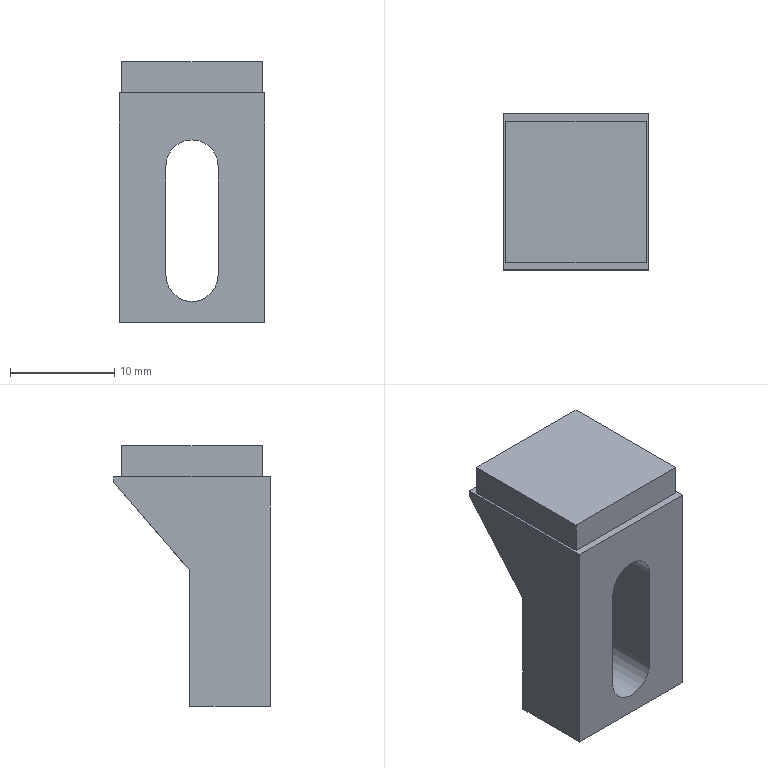Part | SolidWorks | features ICE 4, Extrusion 1 | 1 solid | 24 faces | box 14 x 15 x 25 mm | volume 2645 mm3 | plane 18 | cylinder 6 | commonest cylinder face diameters 5 x3 8.5 x3
STEP:
#1=CARTESIAN_POINT('',(0.,-7.5,-6.));
#2=VERTEX_POINT('',#1);
#3=CARTESIAN_POINT('',(2.5,-7.5,-8.5));
#4=VERTEX_POINT('',#3);
#5=CARTESIAN_POINT('',(0.,-7.5,-8.5));
#6=DIRECTION('',(0.,1.,0.));
#7=DIRECTION('',(0.,0.,1.));
#8=AXIS2_PLACEMENT_3D('',#5,#6,#7);
#9=CIRCLE('',#8,2.5);
#10=EDGE_CURVE('',#2,#4,#9,.T.);
#11=ORIENTED_EDGE('',*,*,#10,.F.);
#12=CARTESIAN_POINT('',(0.,-1.1,-6.));
#13=VERTEX_POINT('',#12);
#14=CARTESIAN_POINT('',(0.,-11.1,-6.));
#15=DIRECTION('',(0.,1.,0.));
#16=VECTOR('',#15,1000.);
#17=LINE('',#14,#16);
#18=EDGE_CURVE('',#2,#13,#17,.T.);
#19=ORIENTED_EDGE('',*,*,#18,.T.);
#20=CARTESIAN_POINT('',(2.5,-1.1,-8.5));
#21=VERTEX_POINT('',#20);
#22=CARTESIAN_POINT('',(0.,-1.1,-8.5));
#23=DIRECTION('',(0.,-1.,0.));
#24=DIRECTION('',(0.,0.,-1.));
#25=AXIS2_PLACEMENT_3D('',#22,#23,#24);
#26=CIRCLE('',#25,2.5);
#27=EDGE_CURVE('',#21,#13,#26,.T.);
#28=ORIENTED_EDGE('',*,*,#27,.F.);
#29=CARTESIAN_POINT('',(2.5,-11.1,-8.5));
#30=DIRECTION('',(0.,1.,0.));
#31=VECTOR('',#30,1000.);
#32=LINE('',#29,#31);
#33=EDGE_CURVE('',#4,#21,#32,.T.);
#34=ORIENTED_EDGE('',*,*,#33,.F.);
#35=EDGE_LOOP('',(#11,#19,#28,#34));
#36=FACE_OUTER_BOUND('',#35,.T.);
#37=CARTESIAN_POINT('',(0.,-11.1,-8.5));
#38=DIRECTION('',(0.,1.,0.));
#39=DIRECTION('',(0.,0.,1.));
#40=AXIS2_PLACEMENT_3D('',#37,#38,#39);
#41=CYLINDRICAL_SURFACE('',#40,2.5);
#42=ADVANCED_FACE('',(#36),#41,.F.);
#43=CARTESIAN_POINT('',(0.,-1.1,-4.25));
#44=VERTEX_POINT('',#43);
#45=CARTESIAN_POINT('',(4.25,-1.1,-8.5));
#46=VERTEX_POINT('',#45);
#47=CARTESIAN_POINT('',(0.,-1.1,-8.5));
#48=DIRECTION('',(0.,1.,0.));
#49=DIRECTION('',(0.,0.,-1.));
#50=AXIS2_PLACEMENT_3D('',#47,#48,#49);
#51=CIRCLE('',#50,4.25);
#52=EDGE_CURVE('',#44,#46,#51,.T.);
#53=ORIENTED_EDGE('',*,*,#52,.F.);
#54=CARTESIAN_POINT('',(0.,5.568,-4.25));
#55=VERTEX_POINT('',#54);
#56=CARTESIAN_POINT('',(0.,-23.215,-4.25));
#57=DIRECTION('',(0.,1.,0.));
#58=VECTOR('',#57,1000.);
#59=LINE('',#56,#58);
#60=EDGE_CURVE('',#44,#55,#59,.T.);
#61=ORIENTED_EDGE('',*,*,#60,.T.);
#62=CARTESIAN_POINT('',(4.25,1.918,-8.5));
#63=VERTEX_POINT('',#62);
#64=CARTESIAN_POINT('',(4.25,1.918,-8.5));
#65=CARTESIAN_POINT('',(4.25,4.056,-6.01));
#66=CARTESIAN_POINT('',(2.49,5.568,-4.25));
#67=CARTESIAN_POINT('',(0.,5.568,-4.25));
#68=(BOUNDED_CURVE()B_SPLINE_CURVE(3,(#64,#65,#66,#67),.UNSPECIFIED.,.F.,.F.)B_SPLINE_CURVE_WITH_KNOTS((4,4),(4.712,6.283),.UNSPECIFIED.)CURVE()GEOMETRIC_REPRESENTATION_ITEM()RATIONAL_B_SPLINE_CURVE((1.,0.8047,0.8047,1.))REPRESENTATION_ITEM(''));
#69=EDGE_CURVE('',#63,#55,#68,.T.);
#70=ORIENTED_EDGE('',*,*,#69,.F.);
#71=CARTESIAN_POINT('',(4.25,-23.215,-8.5));
#72=DIRECTION('',(0.,1.,0.));
#73=VECTOR('',#72,1000.);
#74=LINE('',#71,#73);
#75=EDGE_CURVE('',#46,#63,#74,.T.);
#76=ORIENTED_EDGE('',*,*,#75,.F.);
#77=EDGE_LOOP('',(#53,#61,#70,#76));
#78=FACE_OUTER_BOUND('',#77,.T.);
#79=CARTESIAN_POINT('',(0.,-23.215,-8.5));
#80=DIRECTION('',(0.,1.,0.));
#81=DIRECTION('',(0.,0.,1.));
#82=AXIS2_PLACEMENT_3D('',#79,#80,#81);
#83=CYLINDRICAL_SURFACE('',#82,4.25);
#84=ADVANCED_FACE('',(#78),#83,.F.);
#85=CARTESIAN_POINT('',(6.75,-6.75,-1.5));
#86=VERTEX_POINT('',#85);
#87=CARTESIAN_POINT('',(6.75,6.75,-1.5));
#88=VERTEX_POINT('',#87);
#89=CARTESIAN_POINT('',(6.75,6.75,-1.5));
#90=DIRECTION('',(0.,1.,0.));
#91=VECTOR('',#90,1000.);
#92=LINE('',#89,#91);
#93=EDGE_CURVE('',#86,#88,#92,.T.);
#94=ORIENTED_EDGE('',*,*,#93,.T.);
#95=CARTESIAN_POINT('',(6.75,6.75,1.5));
#96=VERTEX_POINT('',#95);
#97=CARTESIAN_POINT('',(6.75,6.75,1.5));
#98=DIRECTION('',(0.,0.,-1.));
#99=VECTOR('',#98,1000.);
#100=LINE('',#97,#99);
#101=EDGE_CURVE('',#96,#88,#100,.T.);
#102=ORIENTED_EDGE('',*,*,#101,.F.);
#103=CARTESIAN_POINT('',(6.75,-6.75,1.5));
#104=VERTEX_POINT('',#103);
#105=CARTESIAN_POINT('',(6.75,6.75,1.5));
#106=DIRECTION('',(0.,1.,0.));
#107=VECTOR('',#106,1000.);
#108=LINE('',#105,#107);
#109=EDGE_CURVE('',#104,#96,#108,.T.);
#110=ORIENTED_EDGE('',*,*,#109,.F.);
#111=CARTESIAN_POINT('',(6.75,-6.75,1.5));
#112=DIRECTION('',(0.,0.,-1.));
#113=VECTOR('',#112,1000.);
#114=LINE('',#111,#113);
#115=EDGE_CURVE('',#104,#86,#114,.T.);
#116=ORIENTED_EDGE('',*,*,#115,.T.);
#117=EDGE_LOOP('',(#94,#102,#110,#116));
#118=FACE_OUTER_BOUND('',#117,.T.);
#119=CARTESIAN_POINT('',(6.75,6.75,1.5));
#120=DIRECTION('',(-1.,0.,0.));
#121=DIRECTION('',(0.,0.,1.));
#122=AXIS2_PLACEMENT_3D('',#119,#120,#121);
#123=PLANE('',#122);
#124=ADVANCED_FACE('',(#118),#123,.F.);
#125=CARTESIAN_POINT('',(-6.75,6.75,-1.5));
#126=VERTEX_POINT('',#125);
#127=CARTESIAN_POINT('',(-6.75,6.75,-1.5));
#128=DIRECTION('',(-1.,0.,0.));
#129=VECTOR('',#128,1000.);
#130=LINE('',#127,#129);
#131=EDGE_CURVE('',#88,#126,#130,.T.);
#132=ORIENTED_EDGE('',*,*,#131,.T.);
#133=CARTESIAN_POINT('',(-6.75,6.75,1.5));
#134=VERTEX_POINT('',#133);
#135=CARTESIAN_POINT('',(-6.75,6.75,1.5));
#136=DIRECTION('',(0.,0.,-1.));
#137=VECTOR('',#136,1000.);
#138=LINE('',#135,#137);
#139=EDGE_CURVE('',#134,#126,#138,.T.);
#140=ORIENTED_EDGE('',*,*,#139,.F.);
#141=CARTESIAN_POINT('',(-6.75,6.75,1.5));
#142=DIRECTION('',(-1.,0.,0.));
#143=VECTOR('',#142,1000.);
#144=LINE('',#141,#143);
#145=EDGE_CURVE('',#96,#134,#144,.T.);
#146=ORIENTED_EDGE('',*,*,#145,.F.);
#147=ORIENTED_EDGE('',*,*,#101,.T.);
#148=EDGE_LOOP('',(#132,#140,#146,#147));
#149=FACE_OUTER_BOUND('',#148,.T.);
#150=CARTESIAN_POINT('',(-6.75,6.75,1.5));
#151=DIRECTION('',(0.,-1.,0.));
#152=DIRECTION('',(0.,0.,-1.));
#153=AXIS2_PLACEMENT_3D('',#150,#151,#152);
#154=PLANE('',#153);
#155=ADVANCED_FACE('',(#149),#154,.F.);
#156=CARTESIAN_POINT('',(-6.75,-6.75,-1.5));
#157=VERTEX_POINT('',#156);
#158=CARTESIAN_POINT('',(-6.75,6.75,-1.5));
#159=DIRECTION('',(0.,-1.,0.));
#160=VECTOR('',#159,1000.);
#161=LINE('',#158,#160);
#162=EDGE_CURVE('',#126,#157,#161,.T.);
#163=ORIENTED_EDGE('',*,*,#162,.T.);
#164=CARTESIAN_POINT('',(-6.75,-6.75,1.5));
#165=VERTEX_POINT('',#164);
#166=CARTESIAN_POINT('',(-6.75,-6.75,1.5));
#167=DIRECTION('',(0.,0.,-1.));
#168=VECTOR('',#167,1000.);
#169=LINE('',#166,#168);
#170=EDGE_CURVE('',#165,#157,#169,.T.);
#171=ORIENTED_EDGE('',*,*,#170,.F.);
#172=CARTESIAN_POINT('',(-6.75,6.75,1.5));
#173=DIRECTION('',(0.,-1.,0.));
#174=VECTOR('',#173,1000.);
#175=LINE('',#172,#174);
#176=EDGE_CURVE('',#134,#165,#175,.T.);
#177=ORIENTED_EDGE('',*,*,#176,.F.);
#178=ORIENTED_EDGE('',*,*,#139,.T.);
#179=EDGE_LOOP('',(#163,#171,#177,#178));
#180=FACE_OUTER_BOUND('',#179,.T.);
#181=CARTESIAN_POINT('',(-6.75,6.75,1.5));
#182=DIRECTION('',(1.,0.,0.));
#183=DIRECTION('',(0.,0.,-1.));
#184=AXIS2_PLACEMENT_3D('',#181,#182,#183);
#185=PLANE('',#184);
#186=ADVANCED_FACE('',(#180),#185,.F.);
#187=CARTESIAN_POINT('',(-6.75,-6.75,-1.5));
#188=DIRECTION('',(1.,0.,0.));
#189=VECTOR('',#188,1000.);
#190=LINE('',#187,#189);
#191=EDGE_CURVE('',#157,#86,#190,.T.);
#192=ORIENTED_EDGE('',*,*,#191,.T.);
#193=ORIENTED_EDGE('',*,*,#115,.F.);
#194=CARTESIAN_POINT('',(-6.75,-6.75,1.5));
#195=DIRECTION('',(1.,0.,0.));
#196=VECTOR('',#195,1000.);
#197=LINE('',#194,#196);
#198=EDGE_CURVE('',#165,#104,#197,.T.);
#199=ORIENTED_EDGE('',*,*,#198,.F.);
#200=ORIENTED_EDGE('',*,*,#170,.T.);
#201=EDGE_LOOP('',(#192,#193,#199,#200));
#202=FACE_OUTER_BOUND('',#201,.T.);
#203=CARTESIAN_POINT('',(-6.75,-6.75,1.5));
#204=DIRECTION('',(0.,1.,0.));
#205=DIRECTION('',(0.,0.,1.));
#206=AXIS2_PLACEMENT_3D('',#203,#204,#205);
#207=PLANE('',#206);
#208=ADVANCED_FACE('',(#202),#207,.F.);
#209=ORIENTED_EDGE('',*,*,#109,.T.);
#210=ORIENTED_EDGE('',*,*,#145,.T.);
#211=ORIENTED_EDGE('',*,*,#176,.T.);
#212=ORIENTED_EDGE('',*,*,#198,.T.);
#213=EDGE_LOOP('',(#209,#210,#211,#212));
#214=FACE_OUTER_BOUND('',#213,.T.);
#215=CARTESIAN_POINT('',(0.,0.,1.5));
#216=DIRECTION('',(0.,0.,1.));
#217=DIRECTION('',(1.,0.,0.));
#218=AXIS2_PLACEMENT_3D('',#215,#216,#217);
#219=PLANE('',#218);
#220=ADVANCED_FACE('',(#214),#219,.T.);
#221=CARTESIAN_POINT('',(-7.,-7.5,-1.5));
#222=VERTEX_POINT('',#221);
#223=CARTESIAN_POINT('',(-7.,7.5,-1.5));
#224=VERTEX_POINT('',#223);
#225=CARTESIAN_POINT('',(-7.,7.5,-1.5));
#226=DIRECTION('',(0.,1.,0.));
#227=VECTOR('',#226,1000.);
#228=LINE('',#225,#227);
#229=EDGE_CURVE('',#222,#224,#228,.T.);
#230=ORIENTED_EDGE('',*,*,#229,.F.);
#231=CARTESIAN_POINT('',(7.,-7.5,-1.5));
#232=VERTEX_POINT('',#231);
#233=CARTESIAN_POINT('',(7.,-7.5,-1.5));
#234=DIRECTION('',(-1.,0.,0.));
#235=VECTOR('',#234,1000.);
#236=LINE('',#233,#235);
#237=EDGE_CURVE('',#232,#222,#236,.T.);
#238=ORIENTED_EDGE('',*,*,#237,.F.);
#239=CARTESIAN_POINT('',(7.,7.5,-1.5));
#240=VERTEX_POINT('',#239);
#241=CARTESIAN_POINT('',(7.,7.5,-1.5));
#242=DIRECTION('',(0.,-1.,0.));
#243=VECTOR('',#242,1000.);
#244=LINE('',#241,#243);
#245=EDGE_CURVE('',#240,#232,#244,.T.);
#246=ORIENTED_EDGE('',*,*,#245,.F.);
#247=CARTESIAN_POINT('',(7.,7.5,-1.5));
#248=DIRECTION('',(1.,0.,0.));
#249=VECTOR('',#248,1000.);
#250=LINE('',#247,#249);
#251=EDGE_CURVE('',#224,#240,#250,.T.);
#252=ORIENTED_EDGE('',*,*,#251,.F.);
#253=EDGE_LOOP('',(#230,#238,#246,#252));
#254=FACE_OUTER_BOUND('',#253,.T.);
#255=ORIENTED_EDGE('',*,*,#131,.F.);
#256=ORIENTED_EDGE('',*,*,#93,.F.);
#257=ORIENTED_EDGE('',*,*,#191,.F.);
#258=ORIENTED_EDGE('',*,*,#162,.F.);
#259=EDGE_LOOP('',(#255,#256,#257,#258));
#260=FACE_BOUND('',#259,.T.);
#261=CARTESIAN_POINT('',(0.,0.,-1.5));
#262=DIRECTION('',(0.,0.,-1.));
#263=DIRECTION('',(-1.,0.,0.));
#264=AXIS2_PLACEMENT_3D('',#261,#262,#263);
#265=PLANE('',#264);
#266=ADVANCED_FACE('',(#254,#260),#265,.F.);
#267=CARTESIAN_POINT('',(-7.,7.5,-2.));
#268=VERTEX_POINT('',#267);
#269=CARTESIAN_POINT('',(-7.,0.2,-10.5));
#270=VERTEX_POINT('',#269);
#271=CARTESIAN_POINT('',(-7.,-3.127,-14.374));
#272=DIRECTION('',(0.,-0.6515,-0.7586));
#273=VECTOR('',#272,1000.);
#274=LINE('',#271,#273);
#275=EDGE_CURVE('',#268,#270,#274,.T.);
#276=ORIENTED_EDGE('',*,*,#275,.T.);
#277=CARTESIAN_POINT('',(-7.,0.2,-23.5));
#278=VERTEX_POINT('',#277);
#279=CARTESIAN_POINT('',(-7.,0.2,-23.5));
#280=DIRECTION('',(0.,0.,-1.));
#281=VECTOR('',#280,1000.);
#282=LINE('',#279,#281);
#283=EDGE_CURVE('',#270,#278,#282,.T.);
#284=ORIENTED_EDGE('',*,*,#283,.T.);
#285=CARTESIAN_POINT('',(-7.,-7.5,-23.5));
#286=VERTEX_POINT('',#285);
#287=CARTESIAN_POINT('',(-7.,7.5,-23.5));
#288=DIRECTION('',(0.,1.,0.));
#289=VECTOR('',#288,1000.);
#290=LINE('',#287,#289);
#291=EDGE_CURVE('',#286,#278,#290,.T.);
#292=ORIENTED_EDGE('',*,*,#291,.F.);
#293=CARTESIAN_POINT('',(-7.,-7.5,-23.5));
#294=DIRECTION('',(0.,0.,1.));
#295=VECTOR('',#294,1000.);
#296=LINE('',#293,#295);
#297=EDGE_CURVE('',#286,#222,#296,.T.);
#298=ORIENTED_EDGE('',*,*,#297,.T.);
#299=ORIENTED_EDGE('',*,*,#229,.T.);
#300=CARTESIAN_POINT('',(-7.,7.5,-23.5));
#301=DIRECTION('',(0.,0.,1.));
#302=VECTOR('',#301,1000.);
#303=LINE('',#300,#302);
#304=EDGE_CURVE('',#268,#224,#303,.T.);
#305=ORIENTED_EDGE('',*,*,#304,.F.);
#306=EDGE_LOOP('',(#276,#284,#292,#298,#299,#305));
#307=FACE_OUTER_BOUND('',#306,.T.);
#308=CARTESIAN_POINT('',(-7.,7.5,-23.5));
#309=DIRECTION('',(1.,0.,0.));
#310=DIRECTION('',(0.,0.,-1.));
#311=AXIS2_PLACEMENT_3D('',#308,#309,#310);
#312=PLANE('',#311);
#313=ADVANCED_FACE('',(#307),#312,.F.);
#314=CARTESIAN_POINT('',(7.,7.5,-2.));
#315=VERTEX_POINT('',#314);
#316=CARTESIAN_POINT('',(7.,7.5,-23.5));
#317=DIRECTION('',(0.,0.,1.));
#318=VECTOR('',#317,1000.);
#319=LINE('',#316,#318);
#320=EDGE_CURVE('',#315,#240,#319,.T.);
#321=ORIENTED_EDGE('',*,*,#320,.F.);
#322=CARTESIAN_POINT('',(47.74,7.5,-2.));
#323=DIRECTION('',(-1.,0.,0.));
#324=VECTOR('',#323,1000.);
#325=LINE('',#322,#324);
#326=EDGE_CURVE('',#315,#268,#325,.T.);
#327=ORIENTED_EDGE('',*,*,#326,.T.);
#328=ORIENTED_EDGE('',*,*,#304,.T.);
#329=ORIENTED_EDGE('',*,*,#251,.T.);
#330=EDGE_LOOP('',(#321,#327,#328,#329));
#331=FACE_OUTER_BOUND('',#330,.T.);
#332=CARTESIAN_POINT('',(7.,7.5,-23.5));
#333=DIRECTION('',(0.,-1.,0.));
#334=DIRECTION('',(0.,0.,-1.));
#335=AXIS2_PLACEMENT_3D('',#332,#333,#334);
#336=PLANE('',#335);
#337=ADVANCED_FACE('',(#331),#336,.F.);
#338=CARTESIAN_POINT('',(7.,0.2,-23.5));
#339=VERTEX_POINT('',#338);
#340=CARTESIAN_POINT('',(7.,-7.5,-23.5));
#341=VERTEX_POINT('',#340);
#342=CARTESIAN_POINT('',(7.,7.5,-23.5));
#343=DIRECTION('',(0.,-1.,0.));
#344=VECTOR('',#343,1000.);
#345=LINE('',#342,#344);
#346=EDGE_CURVE('',#339,#341,#345,.T.);
#347=ORIENTED_EDGE('',*,*,#346,.F.);
#348=CARTESIAN_POINT('',(7.,0.2,-10.5));
#349=VERTEX_POINT('',#348);
#350=CARTESIAN_POINT('',(7.,0.2,-23.5));
#351=DIRECTION('',(0.,0.,1.));
#352=VECTOR('',#351,1000.);
#353=LINE('',#350,#352);
#354=EDGE_CURVE('',#339,#349,#353,.T.);
#355=ORIENTED_EDGE('',*,*,#354,.T.);
#356=CARTESIAN_POINT('',(7.,-3.127,-14.374));
#357=DIRECTION('',(0.,0.6515,0.7586));
#358=VECTOR('',#357,1000.);
#359=LINE('',#356,#358);
#360=EDGE_CURVE('',#349,#315,#359,.T.);
#361=ORIENTED_EDGE('',*,*,#360,.T.);
#362=ORIENTED_EDGE('',*,*,#320,.T.);
#363=ORIENTED_EDGE('',*,*,#245,.T.);
#364=CARTESIAN_POINT('',(7.,-7.5,-23.5));
#365=DIRECTION('',(0.,0.,1.));
#366=VECTOR('',#365,1000.);
#367=LINE('',#364,#366);
#368=EDGE_CURVE('',#341,#232,#367,.T.);
#369=ORIENTED_EDGE('',*,*,#368,.F.);
#370=EDGE_LOOP('',(#347,#355,#361,#362,#363,#369));
#371=FACE_OUTER_BOUND('',#370,.T.);
#372=CARTESIAN_POINT('',(7.,7.5,-23.5));
#373=DIRECTION('',(-1.,0.,0.));
#374=DIRECTION('',(0.,0.,1.));
#375=AXIS2_PLACEMENT_3D('',#372,#373,#374);
#376=PLANE('',#375);
#377=ADVANCED_FACE('',(#371),#376,.F.);
#378=CARTESIAN_POINT('',(2.5,-7.5,-19.));
#379=VERTEX_POINT('',#378);
#380=CARTESIAN_POINT('',(-2.5,-7.5,-19.));
#381=VERTEX_POINT('',#380);
#382=CARTESIAN_POINT('',(0.,-7.5,-19.));
#383=DIRECTION('',(0.,1.,0.));
#384=DIRECTION('',(0.,0.,1.));
#385=AXIS2_PLACEMENT_3D('',#382,#383,#384);
#386=CIRCLE('',#385,2.5);
#387=EDGE_CURVE('',#379,#381,#386,.T.);
#388=ORIENTED_EDGE('',*,*,#387,.T.);
#389=CARTESIAN_POINT('',(-2.5,-7.5,-8.5));
#390=VERTEX_POINT('',#389);
#391=CARTESIAN_POINT('',(-2.5,-7.5,-23.5));
#392=DIRECTION('',(0.,0.,1.));
#393=VECTOR('',#392,1000.);
#394=LINE('',#391,#393);
#395=EDGE_CURVE('',#381,#390,#394,.T.);
#396=ORIENTED_EDGE('',*,*,#395,.T.);
#397=CARTESIAN_POINT('',(0.,-7.5,-8.5));
#398=DIRECTION('',(0.,1.,0.));
#399=DIRECTION('',(0.,0.,1.));
#400=AXIS2_PLACEMENT_3D('',#397,#398,#399);
#401=CIRCLE('',#400,2.5);
#402=EDGE_CURVE('',#390,#2,#401,.T.);
#403=ORIENTED_EDGE('',*,*,#402,.T.);
#404=ORIENTED_EDGE('',*,*,#10,.T.);
#405=CARTESIAN_POINT('',(2.5,-7.5,-23.5));
#406=DIRECTION('',(0.,0.,1.));
#407=VECTOR('',#406,1000.);
#408=LINE('',#405,#407);
#409=EDGE_CURVE('',#379,#4,#408,.T.);
#410=ORIENTED_EDGE('',*,*,#409,.F.);
#411=EDGE_LOOP('',(#388,#396,#403,#404,#410));
#412=FACE_BOUND('',#411,.T.);
#413=ORIENTED_EDGE('',*,*,#237,.T.);
#414=ORIENTED_EDGE('',*,*,#297,.F.);
#415=CARTESIAN_POINT('',(7.,-7.5,-23.5));
#416=DIRECTION('',(-1.,0.,0.));
#417=VECTOR('',#416,1000.);
#418=LINE('',#415,#417);
#419=EDGE_CURVE('',#341,#286,#418,.T.);
#420=ORIENTED_EDGE('',*,*,#419,.F.);
#421=ORIENTED_EDGE('',*,*,#368,.T.);
#422=EDGE_LOOP('',(#413,#414,#420,#421));
#423=FACE_OUTER_BOUND('',#422,.T.);
#424=CARTESIAN_POINT('',(7.,-7.5,-23.5));
#425=DIRECTION('',(0.,1.,0.));
#426=DIRECTION('',(0.,0.,1.));
#427=AXIS2_PLACEMENT_3D('',#424,#425,#426);
#428=PLANE('',#427);
#429=ADVANCED_FACE('',(#412,#423),#428,.F.);
#430=CARTESIAN_POINT('',(0.,0.2,-23.5));
#431=DIRECTION('',(-1.,0.,0.));
#432=VECTOR('',#431,1000.);
#433=LINE('',#430,#432);
#434=EDGE_CURVE('',#339,#278,#433,.T.);
#435=ORIENTED_EDGE('',*,*,#434,.F.);
#436=ORIENTED_EDGE('',*,*,#346,.T.);
#437=ORIENTED_EDGE('',*,*,#419,.T.);
#438=ORIENTED_EDGE('',*,*,#291,.T.);
#439=EDGE_LOOP('',(#435,#436,#437,#438));
#440=FACE_OUTER_BOUND('',#439,.T.);
#441=CARTESIAN_POINT('',(0.,0.,-23.5));
#442=DIRECTION('',(0.,0.,-1.));
#443=DIRECTION('',(-1.,0.,0.));
#444=AXIS2_PLACEMENT_3D('',#441,#442,#443);
#445=PLANE('',#444);
#446=ADVANCED_FACE('',(#440),#445,.T.);
#447=ORIENTED_EDGE('',*,*,#69,.T.);
#448=CARTESIAN_POINT('',(-4.25,1.918,-8.5));
#449=VERTEX_POINT('',#448);
#450=CARTESIAN_POINT('',(0.,5.568,-4.25));
#451=CARTESIAN_POINT('',(-2.49,5.568,-4.25));
#452=CARTESIAN_POINT('',(-4.25,4.056,-6.01));
#453=CARTESIAN_POINT('',(-4.25,1.918,-8.5));
#454=(BOUNDED_CURVE()B_SPLINE_CURVE(3,(#450,#451,#452,#453),.UNSPECIFIED.,.F.,.F.)B_SPLINE_CURVE_WITH_KNOTS((4,4),(0.,1.571),.UNSPECIFIED.)CURVE()GEOMETRIC_REPRESENTATION_ITEM()RATIONAL_B_SPLINE_CURVE((1.,0.8047,0.8047,1.))REPRESENTATION_ITEM(''));
#455=EDGE_CURVE('',#55,#449,#454,.T.);
#456=ORIENTED_EDGE('',*,*,#455,.T.);
#457=CARTESIAN_POINT('',(-4.25,0.2,-10.5));
#458=VERTEX_POINT('',#457);
#459=CARTESIAN_POINT('',(-4.25,0.2,-10.5));
#460=DIRECTION('',(0.,-0.6515,-0.7586));
#461=VECTOR('',#460,1000.);
#462=LINE('',#459,#461);
#463=EDGE_CURVE('',#449,#458,#462,.T.);
#464=ORIENTED_EDGE('',*,*,#463,.T.);
#465=CARTESIAN_POINT('',(47.74,0.2,-10.5));
#466=DIRECTION('',(-1.,0.,0.));
#467=VECTOR('',#466,1000.);
#468=LINE('',#465,#467);
#469=EDGE_CURVE('',#458,#270,#468,.T.);
#470=ORIENTED_EDGE('',*,*,#469,.T.);
#471=ORIENTED_EDGE('',*,*,#275,.F.);
#472=ORIENTED_EDGE('',*,*,#326,.F.);
#473=ORIENTED_EDGE('',*,*,#360,.F.);
#474=CARTESIAN_POINT('',(4.25,0.2,-10.5));
#475=VERTEX_POINT('',#474);
#476=CARTESIAN_POINT('',(47.74,0.2,-10.5));
#477=DIRECTION('',(-1.,0.,0.));
#478=VECTOR('',#477,1000.);
#479=LINE('',#476,#478);
#480=EDGE_CURVE('',#349,#475,#479,.T.);
#481=ORIENTED_EDGE('',*,*,#480,.T.);
#482=CARTESIAN_POINT('',(4.25,0.2,-10.5));
#483=DIRECTION('',(0.,-0.6515,-0.7586));
#484=VECTOR('',#483,1000.);
#485=LINE('',#482,#484);
#486=EDGE_CURVE('',#63,#475,#485,.T.);
#487=ORIENTED_EDGE('',*,*,#486,.F.);
#488=EDGE_LOOP('',(#447,#456,#464,#470,#471,#472,#473,#481,#487));
#489=FACE_OUTER_BOUND('',#488,.T.);
#490=CARTESIAN_POINT('',(47.74,0.2,-10.5));
#491=DIRECTION('',(0.,-0.7586,0.6515));
#492=DIRECTION('',(0.,-0.6515,-0.7586));
#493=AXIS2_PLACEMENT_3D('',#490,#491,#492);
#494=PLANE('',#493);
#495=ADVANCED_FACE('',(#489),#494,.F.);
#496=ORIENTED_EDGE('',*,*,#469,.F.);
#497=CARTESIAN_POINT('',(-4.25,0.2,-19.));
#498=VERTEX_POINT('',#497);
#499=CARTESIAN_POINT('',(-4.25,0.2,-23.5));
#500=DIRECTION('',(0.,0.,-1.));
#501=VECTOR('',#500,1000.);
#502=LINE('',#499,#501);
#503=EDGE_CURVE('',#458,#498,#502,.T.);
#504=ORIENTED_EDGE('',*,*,#503,.T.);
#505=CARTESIAN_POINT('',(4.25,0.2,-19.));
#506=VERTEX_POINT('',#505);
#507=CARTESIAN_POINT('',(0.,0.2,-19.));
#508=DIRECTION('',(0.,-1.,0.));
#509=DIRECTION('',(0.,0.,-1.));
#510=AXIS2_PLACEMENT_3D('',#507,#508,#509);
#511=CIRCLE('',#510,4.25);
#512=EDGE_CURVE('',#498,#506,#511,.T.);
#513=ORIENTED_EDGE('',*,*,#512,.T.);
#514=CARTESIAN_POINT('',(4.25,0.2,-23.5));
#515=DIRECTION('',(0.,0.,-1.));
#516=VECTOR('',#515,1000.);
#517=LINE('',#514,#516);
#518=EDGE_CURVE('',#475,#506,#517,.T.);
#519=ORIENTED_EDGE('',*,*,#518,.F.);
#520=ORIENTED_EDGE('',*,*,#480,.F.);
#521=ORIENTED_EDGE('',*,*,#354,.F.);
#522=ORIENTED_EDGE('',*,*,#434,.T.);
#523=ORIENTED_EDGE('',*,*,#283,.F.);
#524=EDGE_LOOP('',(#496,#504,#513,#519,#520,#521,#522,#523));
#525=FACE_OUTER_BOUND('',#524,.T.);
#526=CARTESIAN_POINT('',(47.74,0.2,-23.5));
#527=DIRECTION('',(0.,-1.,0.));
#528=DIRECTION('',(0.,0.,-1.));
#529=AXIS2_PLACEMENT_3D('',#526,#527,#528);
#530=PLANE('',#529);
#531=ADVANCED_FACE('',(#525),#530,.F.);
#532=ORIENTED_EDGE('',*,*,#60,.F.);
#533=CARTESIAN_POINT('',(-4.25,-1.1,-8.5));
#534=VERTEX_POINT('',#533);
#535=CARTESIAN_POINT('',(0.,-1.1,-8.5));
#536=DIRECTION('',(0.,1.,0.));
#537=DIRECTION('',(0.,0.,-1.));
#538=AXIS2_PLACEMENT_3D('',#535,#536,#537);
#539=CIRCLE('',#538,4.25);
#540=EDGE_CURVE('',#534,#44,#539,.T.);
#541=ORIENTED_EDGE('',*,*,#540,.F.);
#542=CARTESIAN_POINT('',(-4.25,-23.215,-8.5));
#543=DIRECTION('',(0.,1.,0.));
#544=VECTOR('',#543,1000.);
#545=LINE('',#542,#544);
#546=EDGE_CURVE('',#534,#449,#545,.T.);
#547=ORIENTED_EDGE('',*,*,#546,.T.);
#548=ORIENTED_EDGE('',*,*,#455,.F.);
#549=EDGE_LOOP('',(#532,#541,#547,#548));
#550=FACE_OUTER_BOUND('',#549,.T.);
#551=CARTESIAN_POINT('',(0.,-23.215,-8.5));
#552=DIRECTION('',(0.,1.,0.));
#553=DIRECTION('',(0.,0.,1.));
#554=AXIS2_PLACEMENT_3D('',#551,#552,#553);
#555=CYLINDRICAL_SURFACE('',#554,4.25);
#556=ADVANCED_FACE('',(#550),#555,.F.);
#557=ORIENTED_EDGE('',*,*,#546,.F.);
#558=CARTESIAN_POINT('',(-4.25,-1.1,-19.));
#559=VERTEX_POINT('',#558);
#560=CARTESIAN_POINT('',(-4.25,-1.1,-19.));
#561=DIRECTION('',(0.,0.,1.));
#562=VECTOR('',#561,1000.);
#563=LINE('',#560,#562);
#564=EDGE_CURVE('',#559,#534,#563,.T.);
#565=ORIENTED_EDGE('',*,*,#564,.F.);
#566=CARTESIAN_POINT('',(-4.25,-23.215,-19.));
#567=DIRECTION('',(0.,1.,0.));
#568=VECTOR('',#567,1000.);
#569=LINE('',#566,#568);
#570=EDGE_CURVE('',#559,#498,#569,.T.);
#571=ORIENTED_EDGE('',*,*,#570,.T.);
#572=ORIENTED_EDGE('',*,*,#503,.F.);
#573=ORIENTED_EDGE('',*,*,#463,.F.);
#574=EDGE_LOOP('',(#557,#565,#571,#572,#573));
#575=FACE_OUTER_BOUND('',#574,.T.);
#576=CARTESIAN_POINT('',(-4.25,-23.215,-19.));
#577=DIRECTION('',(-1.,0.,0.));
#578=DIRECTION('',(0.,0.,1.));
#579=AXIS2_PLACEMENT_3D('',#576,#577,#578);
#580=PLANE('',#579);
#581=ADVANCED_FACE('',(#575),#580,.F.);
#582=ORIENTED_EDGE('',*,*,#486,.T.);
#583=ORIENTED_EDGE('',*,*,#518,.T.);
#584=CARTESIAN_POINT('',(4.25,-1.1,-19.));
#585=VERTEX_POINT('',#584);
#586=CARTESIAN_POINT('',(4.25,-23.215,-19.));
#587=DIRECTION('',(0.,1.,0.));
#588=VECTOR('',#587,1000.);
#589=LINE('',#586,#588);
#590=EDGE_CURVE('',#585,#506,#589,.T.);
#591=ORIENTED_EDGE('',*,*,#590,.F.);
#592=CARTESIAN_POINT('',(4.25,-1.1,-19.));
#593=DIRECTION('',(0.,0.,1.));
#594=VECTOR('',#593,1000.);
#595=LINE('',#592,#594);
#596=EDGE_CURVE('',#585,#46,#595,.T.);
#597=ORIENTED_EDGE('',*,*,#596,.T.);
#598=ORIENTED_EDGE('',*,*,#75,.T.);
#599=EDGE_LOOP('',(#582,#583,#591,#597,#598));
#600=FACE_OUTER_BOUND('',#599,.T.);
#601=CARTESIAN_POINT('',(4.25,-23.215,-19.));
#602=DIRECTION('',(-1.,0.,0.));
#603=DIRECTION('',(0.,0.,1.));
#604=AXIS2_PLACEMENT_3D('',#601,#602,#603);
#605=PLANE('',#604);
#606=ADVANCED_FACE('',(#600),#605,.T.);
#607=ORIENTED_EDGE('',*,*,#570,.F.);
#608=CARTESIAN_POINT('',(0.,-1.1,-19.));
#609=DIRECTION('',(0.,1.,0.));
#610=DIRECTION('',(0.,0.,-1.));
#611=AXIS2_PLACEMENT_3D('',#608,#609,#610);
#612=CIRCLE('',#611,4.25);
#613=EDGE_CURVE('',#585,#559,#612,.T.);
#614=ORIENTED_EDGE('',*,*,#613,.F.);
#615=ORIENTED_EDGE('',*,*,#590,.T.);
#616=ORIENTED_EDGE('',*,*,#512,.F.);
#617=EDGE_LOOP('',(#607,#614,#615,#616));
#618=FACE_OUTER_BOUND('',#617,.T.);
#619=CARTESIAN_POINT('',(0.,-23.215,-19.));
#620=DIRECTION('',(0.,1.,0.));
#621=DIRECTION('',(0.,0.,1.));
#622=AXIS2_PLACEMENT_3D('',#619,#620,#621);
#623=CYLINDRICAL_SURFACE('',#622,4.25);
#624=ADVANCED_FACE('',(#618),#623,.F.);
#625=ORIENTED_EDGE('',*,*,#27,.T.);
#626=CARTESIAN_POINT('',(-2.5,-1.1,-8.5));
#627=VERTEX_POINT('',#626);
#628=CARTESIAN_POINT('',(0.,-1.1,-8.5));
#629=DIRECTION('',(0.,-1.,0.));
#630=DIRECTION('',(0.,0.,-1.));
#631=AXIS2_PLACEMENT_3D('',#628,#629,#630);
#632=CIRCLE('',#631,2.5);
#633=EDGE_CURVE('',#13,#627,#632,.T.);
#634=ORIENTED_EDGE('',*,*,#633,.T.);
#635=CARTESIAN_POINT('',(-2.5,-1.1,-19.));
#636=VERTEX_POINT('',#635);
#637=CARTESIAN_POINT('',(-2.5,-1.1,-23.5));
#638=DIRECTION('',(0.,0.,-1.));
#639=VECTOR('',#638,1000.);
#640=LINE('',#637,#639);
#641=EDGE_CURVE('',#627,#636,#640,.T.);
#642=ORIENTED_EDGE('',*,*,#641,.T.);
#643=CARTESIAN_POINT('',(2.5,-1.1,-19.));
#644=VERTEX_POINT('',#643);
#645=CARTESIAN_POINT('',(0.,-1.1,-19.));
#646=DIRECTION('',(0.,-1.,0.));
#647=DIRECTION('',(0.,0.,-1.));
#648=AXIS2_PLACEMENT_3D('',#645,#646,#647);
#649=CIRCLE('',#648,2.5);
#650=EDGE_CURVE('',#636,#644,#649,.T.);
#651=ORIENTED_EDGE('',*,*,#650,.T.);
#652=CARTESIAN_POINT('',(2.5,-1.1,-23.5));
#653=DIRECTION('',(0.,0.,-1.));
#654=VECTOR('',#653,1000.);
#655=LINE('',#652,#654);
#656=EDGE_CURVE('',#21,#644,#655,.T.);
#657=ORIENTED_EDGE('',*,*,#656,.F.);
#658=EDGE_LOOP('',(#625,#634,#642,#651,#657));
#659=FACE_BOUND('',#658,.T.);
#660=ORIENTED_EDGE('',*,*,#613,.T.);
#661=ORIENTED_EDGE('',*,*,#564,.T.);
#662=ORIENTED_EDGE('',*,*,#540,.T.);
#663=ORIENTED_EDGE('',*,*,#52,.T.);
#664=ORIENTED_EDGE('',*,*,#596,.F.);
#665=EDGE_LOOP('',(#660,#661,#662,#663,#664));
#666=FACE_OUTER_BOUND('',#665,.T.);
#667=CARTESIAN_POINT('',(47.74,-1.1,-23.5));
#668=DIRECTION('',(0.,-1.,0.));
#669=DIRECTION('',(0.,0.,-1.));
#670=AXIS2_PLACEMENT_3D('',#667,#668,#669);
#671=PLANE('',#670);
#672=ADVANCED_FACE('',(#659,#666),#671,.F.);
#673=CARTESIAN_POINT('',(-2.5,-11.1,-19.));
#674=DIRECTION('',(0.,1.,0.));
#675=VECTOR('',#674,1000.);
#676=LINE('',#673,#675);
#677=EDGE_CURVE('',#381,#636,#676,.T.);
#678=ORIENTED_EDGE('',*,*,#677,.T.);
#679=ORIENTED_EDGE('',*,*,#641,.F.);
#680=CARTESIAN_POINT('',(-2.5,-11.1,-8.5));
#681=DIRECTION('',(0.,1.,0.));
#682=VECTOR('',#681,1000.);
#683=LINE('',#680,#682);
#684=EDGE_CURVE('',#390,#627,#683,.T.);
#685=ORIENTED_EDGE('',*,*,#684,.F.);
#686=ORIENTED_EDGE('',*,*,#395,.F.);
#687=EDGE_LOOP('',(#678,#679,#685,#686));
#688=FACE_OUTER_BOUND('',#687,.T.);
#689=CARTESIAN_POINT('',(-2.5,-11.1,-19.));
#690=DIRECTION('',(-1.,0.,0.));
#691=DIRECTION('',(0.,0.,1.));
#692=AXIS2_PLACEMENT_3D('',#689,#690,#691);
#693=PLANE('',#692);
#694=ADVANCED_FACE('',(#688),#693,.F.);
#695=CARTESIAN_POINT('',(2.5,-11.1,-19.));
#696=DIRECTION('',(0.,1.,0.));
#697=VECTOR('',#696,1000.);
#698=LINE('',#695,#697);
#699=EDGE_CURVE('',#379,#644,#698,.T.);
#700=ORIENTED_EDGE('',*,*,#699,.T.);
#701=ORIENTED_EDGE('',*,*,#650,.F.);
#702=ORIENTED_EDGE('',*,*,#677,.F.);
#703=ORIENTED_EDGE('',*,*,#387,.F.);
#704=EDGE_LOOP('',(#700,#701,#702,#703));
#705=FACE_OUTER_BOUND('',#704,.T.);
#706=CARTESIAN_POINT('',(0.,-11.1,-19.));
#707=DIRECTION('',(0.,1.,0.));
#708=DIRECTION('',(0.,0.,1.));
#709=AXIS2_PLACEMENT_3D('',#706,#707,#708);
#710=CYLINDRICAL_SURFACE('',#709,2.5);
#711=ADVANCED_FACE('',(#705),#710,.F.);
#712=ORIENTED_EDGE('',*,*,#409,.T.);
#713=ORIENTED_EDGE('',*,*,#33,.T.);
#714=ORIENTED_EDGE('',*,*,#656,.T.);
#715=ORIENTED_EDGE('',*,*,#699,.F.);
#716=EDGE_LOOP('',(#712,#713,#714,#715));
#717=FACE_OUTER_BOUND('',#716,.T.);
#718=CARTESIAN_POINT('',(2.5,-11.1,-19.));
#719=DIRECTION('',(-1.,0.,0.));
#720=DIRECTION('',(0.,0.,1.));
#721=AXIS2_PLACEMENT_3D('',#718,#719,#720);
#722=PLANE('',#721);
#723=ADVANCED_FACE('',(#717),#722,.T.);
#724=ORIENTED_EDGE('',*,*,#18,.F.);
#725=ORIENTED_EDGE('',*,*,#402,.F.);
#726=ORIENTED_EDGE('',*,*,#684,.T.);
#727=ORIENTED_EDGE('',*,*,#633,.F.);
#728=EDGE_LOOP('',(#724,#725,#726,#727));
#729=FACE_OUTER_BOUND('',#728,.T.);
#730=CARTESIAN_POINT('',(0.,-11.1,-8.5));
#731=DIRECTION('',(0.,1.,0.));
#732=DIRECTION('',(0.,0.,1.));
#733=AXIS2_PLACEMENT_3D('',#730,#731,#732);
#734=CYLINDRICAL_SURFACE('',#733,2.5);
#735=ADVANCED_FACE('',(#729),#734,.F.);
#736=CLOSED_SHELL('',(#42,#84,#124,#155,#186,#208,#220,#266,#313,#337,#377,#429,#446,#495,#531,#556,#581,#606,#624,#672,#694,#711,#723,#735));
#737=MANIFOLD_SOLID_BREP('',#736);
#738=CARTESIAN_POINT('',(0.,0.,0.));
#739=DIRECTION('',(0.,0.,1.));
#740=DIRECTION('',(1.,0.,0.));
#741=AXIS2_PLACEMENT_3D('',#738,#739,#740);
#742=(LENGTH_UNIT()NAMED_UNIT(*)SI_UNIT(.MILLI.,.METRE.));
#743=UNCERTAINTY_MEASURE_WITH_UNIT(LENGTH_MEASURE(0.00001),#742,'','');
#744=(NAMED_UNIT(*)PLANE_ANGLE_UNIT()SI_UNIT($,.RADIAN.));
#745=(NAMED_UNIT(*)SI_UNIT($,.STERADIAN.)SOLID_ANGLE_UNIT());
#746=(GEOMETRIC_REPRESENTATION_CONTEXT(3)GLOBAL_UNCERTAINTY_ASSIGNED_CONTEXT((#743))GLOBAL_UNIT_ASSIGNED_CONTEXT((#742,#744,#745))REPRESENTATION_CONTEXT('',''));
#747=ADVANCED_BREP_SHAPE_REPRESENTATION('',(#737,#741),#746);